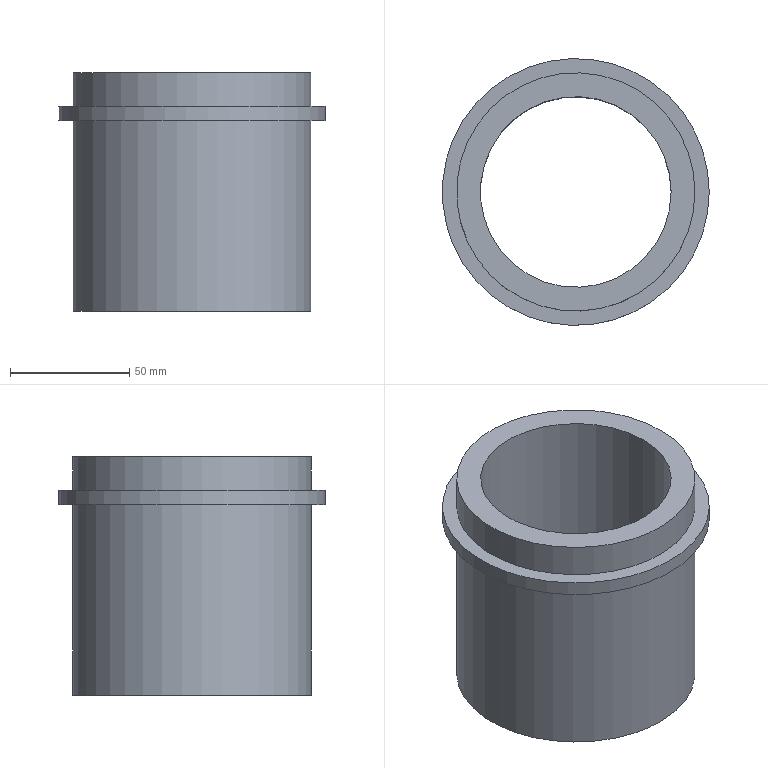Part | NX | features MAIN_BODY 2 | 1 solid | 8 faces | box 112 x 112 x 100 mm | volume 294732 mm3 | plane 4 | cylinder 4 | commonest cylinder face diameters 100 x2 80 x1 112 x1
STEP:
#1=CARTESIAN_POINT('',(-245.,-285.,280.));
#2=VERTEX_POINT('',#1);
#3=CARTESIAN_POINT('',(-295.,-285.,280.));
#4=DIRECTION('',(0.,0.,1.));
#5=DIRECTION('',(1.,0.,0.));
#6=AXIS2_PLACEMENT_3D('',#3,#4,#5);
#7=CIRCLE('',#6,50.);
#8=EDGE_CURVE('',#2,#2,#7,.F.);
#9=ORIENTED_EDGE('',*,*,#8,.F.);
#10=EDGE_LOOP('',(#9));
#11=FACE_BOUND('',#10,.T.);
#12=CARTESIAN_POINT('',(-255.,-285.,280.));
#13=VERTEX_POINT('',#12);
#14=CARTESIAN_POINT('',(-295.,-285.,280.));
#15=DIRECTION('',(0.,0.,1.));
#16=DIRECTION('',(1.,0.,0.));
#17=AXIS2_PLACEMENT_3D('',#14,#15,#16);
#18=CIRCLE('',#17,40.);
#19=EDGE_CURVE('',#13,#13,#18,.F.);
#20=ORIENTED_EDGE('',*,*,#19,.T.);
#21=EDGE_LOOP('',(#20));
#22=FACE_BOUND('',#21,.T.);
#23=CARTESIAN_POINT('',(-295.,-285.,280.));
#24=DIRECTION('',(0.,0.,-1.));
#25=DIRECTION('',(-0.1736,-0.9848,0.));
#26=AXIS2_PLACEMENT_3D('',#23,#24,#25);
#27=PLANE('',#26);
#28=ADVANCED_FACE('',(#11,#22),#27,.F.);
#29=CARTESIAN_POINT('',(-255.,-285.,180.));
#30=VERTEX_POINT('',#29);
#31=CARTESIAN_POINT('',(-295.,-285.,180.));
#32=DIRECTION('',(0.,0.,1.));
#33=DIRECTION('',(1.,0.,0.));
#34=AXIS2_PLACEMENT_3D('',#31,#32,#33);
#35=CIRCLE('',#34,40.);
#36=EDGE_CURVE('',#30,#30,#35,.F.);
#37=ORIENTED_EDGE('',*,*,#36,.F.);
#38=EDGE_LOOP('',(#37));
#39=FACE_BOUND('',#38,.T.);
#40=CARTESIAN_POINT('',(-245.,-285.,180.));
#41=VERTEX_POINT('',#40);
#42=CARTESIAN_POINT('',(-295.,-285.,180.));
#43=DIRECTION('',(0.,0.,1.));
#44=DIRECTION('',(1.,0.,0.));
#45=AXIS2_PLACEMENT_3D('',#42,#43,#44);
#46=CIRCLE('',#45,50.);
#47=EDGE_CURVE('',#41,#41,#46,.F.);
#48=ORIENTED_EDGE('',*,*,#47,.T.);
#49=EDGE_LOOP('',(#48));
#50=FACE_BOUND('',#49,.T.);
#51=CARTESIAN_POINT('',(-295.,-285.,180.));
#52=DIRECTION('',(0.,0.,-1.));
#53=DIRECTION('',(-0.1736,-0.9848,0.));
#54=AXIS2_PLACEMENT_3D('',#51,#52,#53);
#55=PLANE('',#54);
#56=ADVANCED_FACE('',(#39,#50),#55,.T.);
#57=ORIENTED_EDGE('',*,*,#47,.F.);
#58=EDGE_LOOP('',(#57));
#59=FACE_BOUND('',#58,.T.);
#60=CARTESIAN_POINT('',(-245.,-285.,260.));
#61=VERTEX_POINT('',#60);
#62=CARTESIAN_POINT('',(-295.,-285.,260.));
#63=DIRECTION('',(0.,0.,1.));
#64=DIRECTION('',(1.,0.,0.));
#65=AXIS2_PLACEMENT_3D('',#62,#63,#64);
#66=CIRCLE('',#65,50.);
#67=EDGE_CURVE('',#61,#61,#66,.T.);
#68=ORIENTED_EDGE('',*,*,#67,.F.);
#69=EDGE_LOOP('',(#68));
#70=FACE_BOUND('',#69,.T.);
#71=CARTESIAN_POINT('',(-295.,-285.,264.));
#72=DIRECTION('',(0.,0.,-1.));
#73=DIRECTION('',(-0.1736,-0.9848,0.));
#74=AXIS2_PLACEMENT_3D('',#71,#72,#73);
#75=CYLINDRICAL_SURFACE('',#74,50.);
#76=ADVANCED_FACE('',(#59,#70),#75,.T.);
#77=CARTESIAN_POINT('',(-239.,-285.,266.));
#78=VERTEX_POINT('',#77);
#79=CARTESIAN_POINT('',(-295.,-285.,266.));
#80=DIRECTION('',(0.,0.,1.));
#81=DIRECTION('',(1.,0.,0.));
#82=AXIS2_PLACEMENT_3D('',#79,#80,#81);
#83=CIRCLE('',#82,56.);
#84=EDGE_CURVE('',#78,#78,#83,.F.);
#85=ORIENTED_EDGE('',*,*,#84,.T.);
#86=EDGE_LOOP('',(#85));
#87=FACE_BOUND('',#86,.T.);
#88=CARTESIAN_POINT('',(-239.,-285.,260.));
#89=VERTEX_POINT('',#88);
#90=CARTESIAN_POINT('',(-295.,-285.,260.));
#91=DIRECTION('',(0.,0.,1.));
#92=DIRECTION('',(1.,0.,0.));
#93=AXIS2_PLACEMENT_3D('',#90,#91,#92);
#94=CIRCLE('',#93,56.);
#95=EDGE_CURVE('',#89,#89,#94,.F.);
#96=ORIENTED_EDGE('',*,*,#95,.F.);
#97=EDGE_LOOP('',(#96));
#98=FACE_BOUND('',#97,.T.);
#99=CARTESIAN_POINT('',(-295.,-285.,270.));
#100=DIRECTION('',(0.,0.,-1.));
#101=DIRECTION('',(-0.1736,-0.9848,0.));
#102=AXIS2_PLACEMENT_3D('',#99,#100,#101);
#103=CYLINDRICAL_SURFACE('',#102,56.);
#104=ADVANCED_FACE('',(#87,#98),#103,.T.);
#105=ORIENTED_EDGE('',*,*,#67,.T.);
#106=EDGE_LOOP('',(#105));
#107=FACE_BOUND('',#106,.T.);
#108=ORIENTED_EDGE('',*,*,#95,.T.);
#109=EDGE_LOOP('',(#108));
#110=FACE_BOUND('',#109,.T.);
#111=CARTESIAN_POINT('',(-295.,-285.,260.));
#112=DIRECTION('',(0.,0.,-1.));
#113=DIRECTION('',(-0.1736,-0.9848,0.));
#114=AXIS2_PLACEMENT_3D('',#111,#112,#113);
#115=PLANE('',#114);
#116=ADVANCED_FACE('',(#107,#110),#115,.T.);
#117=CARTESIAN_POINT('',(-245.,-285.,266.));
#118=VERTEX_POINT('',#117);
#119=CARTESIAN_POINT('',(-295.,-285.,266.));
#120=DIRECTION('',(0.,0.,1.));
#121=DIRECTION('',(1.,0.,0.));
#122=AXIS2_PLACEMENT_3D('',#119,#120,#121);
#123=CIRCLE('',#122,50.);
#124=EDGE_CURVE('',#118,#118,#123,.T.);
#125=ORIENTED_EDGE('',*,*,#124,.T.);
#126=EDGE_LOOP('',(#125));
#127=FACE_BOUND('',#126,.T.);
#128=ORIENTED_EDGE('',*,*,#8,.T.);
#129=EDGE_LOOP('',(#128));
#130=FACE_BOUND('',#129,.T.);
#131=CARTESIAN_POINT('',(-295.,-285.,277.));
#132=DIRECTION('',(0.,0.,-1.));
#133=DIRECTION('',(-0.1736,-0.9848,0.));
#134=AXIS2_PLACEMENT_3D('',#131,#132,#133);
#135=CYLINDRICAL_SURFACE('',#134,50.);
#136=ADVANCED_FACE('',(#127,#130),#135,.T.);
#137=ORIENTED_EDGE('',*,*,#19,.F.);
#138=EDGE_LOOP('',(#137));
#139=FACE_BOUND('',#138,.T.);
#140=ORIENTED_EDGE('',*,*,#36,.T.);
#141=EDGE_LOOP('',(#140));
#142=FACE_BOUND('',#141,.T.);
#143=CARTESIAN_POINT('',(-295.,-285.,214.));
#144=DIRECTION('',(0.,0.,1.));
#145=DIRECTION('',(0.1736,0.9848,0.));
#146=AXIS2_PLACEMENT_3D('',#143,#144,#145);
#147=CYLINDRICAL_SURFACE('',#146,40.);
#148=ADVANCED_FACE('',(#139,#142),#147,.F.);
#149=ORIENTED_EDGE('',*,*,#84,.F.);
#150=EDGE_LOOP('',(#149));
#151=FACE_BOUND('',#150,.T.);
#152=ORIENTED_EDGE('',*,*,#124,.F.);
#153=EDGE_LOOP('',(#152));
#154=FACE_BOUND('',#153,.T.);
#155=CARTESIAN_POINT('',(-295.,-285.,266.));
#156=DIRECTION('',(0.,0.,-1.));
#157=DIRECTION('',(-0.1736,-0.9848,0.));
#158=AXIS2_PLACEMENT_3D('',#155,#156,#157);
#159=PLANE('',#158);
#160=ADVANCED_FACE('',(#151,#154),#159,.F.);
#161=CLOSED_SHELL('',(#28,#56,#76,#104,#116,#136,#148,#160));
#162=MANIFOLD_SOLID_BREP('',#161);
#163=(LENGTH_UNIT()NAMED_UNIT(*)SI_UNIT(.MILLI.,.METRE.));
#164=UNCERTAINTY_MEASURE_WITH_UNIT(LENGTH_MEASURE(0.00001),#163,'','');
#165=(NAMED_UNIT(*)PLANE_ANGLE_UNIT()SI_UNIT($,.RADIAN.));
#166=(NAMED_UNIT(*)SI_UNIT($,.STERADIAN.)SOLID_ANGLE_UNIT());
#167=(GEOMETRIC_REPRESENTATION_CONTEXT(3)GLOBAL_UNCERTAINTY_ASSIGNED_CONTEXT((#164))GLOBAL_UNIT_ASSIGNED_CONTEXT((#163,#165,#166))REPRESENTATION_CONTEXT('',''));
#168=ADVANCED_BREP_SHAPE_REPRESENTATION('',(#162),#167);